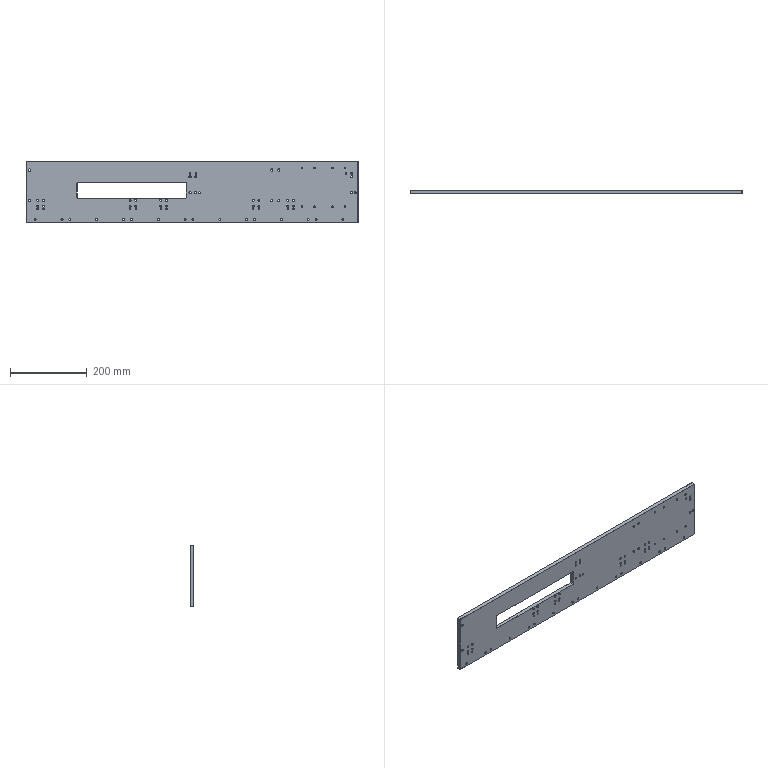Part | NX | 1 solid | 341 faces | box 863 x 10 x 159 mm | volume 1223174 mm3 | cylinder 160 | cone 140 | plane 41 | commonest cylinder face diameters 5 x76 4 x32 3.3 x16 5.5 x12 6 x12 10 x12